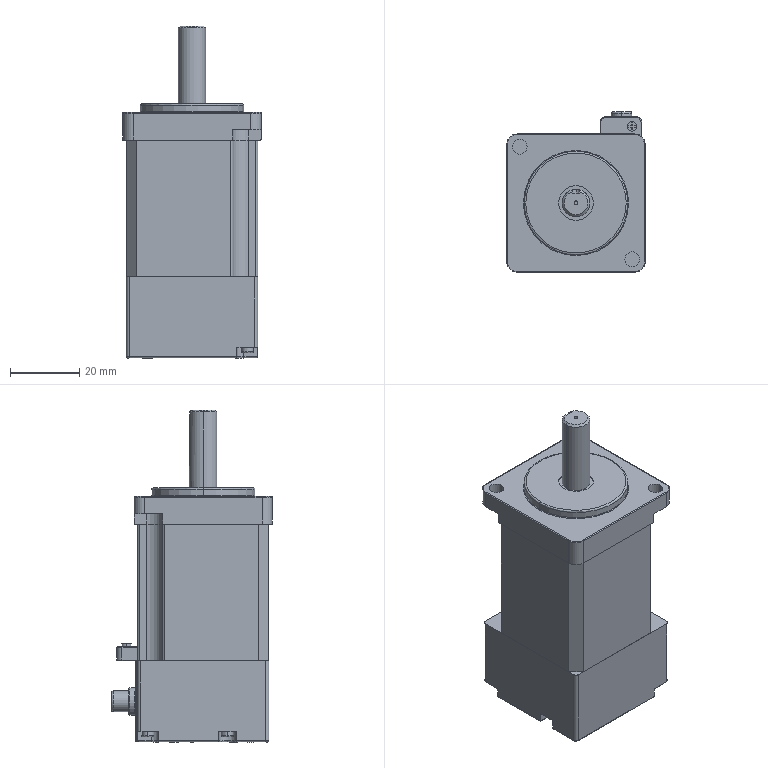Part | SolidWorks | features BaseBody 5 | 5 solids | 257 faces | box 40 x 46.5 x 96 mm | volume 102158 mm3 | plane 134 | cylinder 87 | spline 33 | cone 3 | commonest cylinder face diameters 0.6 x17 0.4 x12 8 x12 3.5 x8 6 x6 2 x5